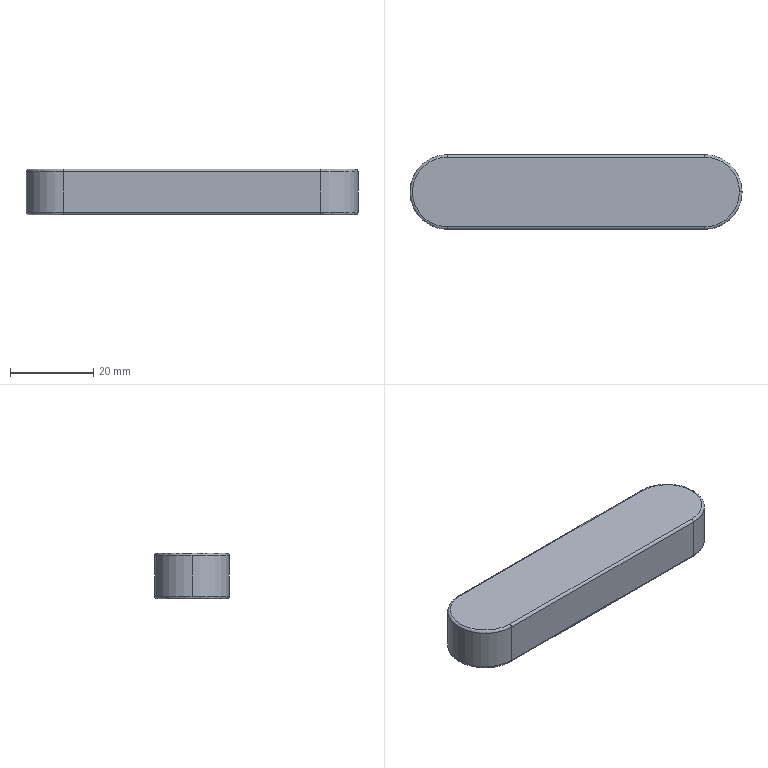Part | STEP file | 1 solid | 17 faces | box 80 x 18 x 11 mm | volume 15047 mm3 | cylinder 7 | spline 6 | plane 4 | commonest cylinder face diameters 1.2 x4 18 x3